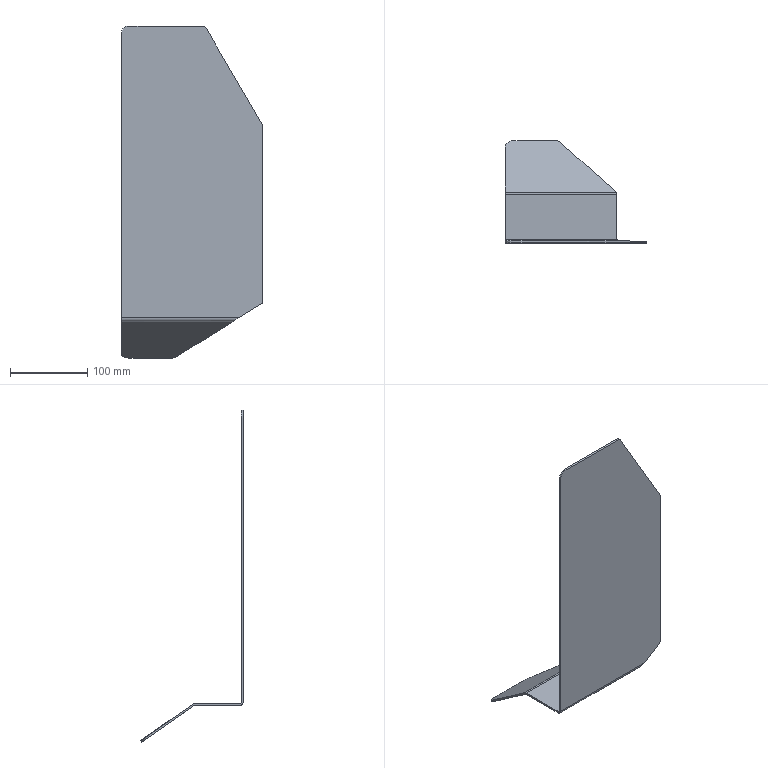Part | SolidWorks | features Fillet 2, FlatPattern 1, ICE 1, SMBaseFlange 1, SheetMetal 1 | 1 solid | 30 faces | box 183 x 132.321 x 429 mm | volume 188831 mm3 | plane 18 | cylinder 10 | spline 2 | commonest cylinder face diameters 10 x4 5 x2 9.6 x2 20 x2
STEP:
#1=CARTESIAN_POINT('',(-24.691,131.,-429.));
#2=VERTEX_POINT('',#1);
#3=CARTESIAN_POINT('',(-81.5,131.,-429.));
#4=VERTEX_POINT('',#3);
#5=CARTESIAN_POINT('',(91.5,131.,-429.));
#6=DIRECTION('',(-1.,0.,0.));
#7=VECTOR('',#6,1000.);
#8=LINE('',#5,#7);
#9=EDGE_CURVE('',#2,#4,#8,.T.);
#10=ORIENTED_EDGE('',*,*,#9,.F.);
#11=CARTESIAN_POINT('',(-21.015,129.681,-428.075));
#12=VERTEX_POINT('',#11);
#13=CARTESIAN_POINT('',(-24.691,126.907,-426.129));
#14=DIRECTION('',(0.,-0.5743,-0.8187));
#15=DIRECTION('',(0.,-0.8187,0.5743));
#16=AXIS2_PLACEMENT_3D('',#13,#14,#15);
#17=CIRCLE('',#16,5.);
#18=EDGE_CURVE('',#2,#12,#17,.T.);
#19=ORIENTED_EDGE('',*,*,#18,.T.);
#20=CARTESIAN_POINT('',(52.237,64.646,-382.453));
#21=VERTEX_POINT('',#20);
#22=CARTESIAN_POINT('',(70.673,48.278,-370.971));
#23=DIRECTION('',(0.6779,-0.6018,0.4222));
#24=VECTOR('',#23,1000.);
#25=LINE('',#22,#24);
#26=EDGE_CURVE('',#12,#21,#25,.T.);
#27=ORIENTED_EDGE('',*,*,#26,.T.);
#28=CARTESIAN_POINT('',(-91.5,64.646,-382.453));
#29=VERTEX_POINT('',#28);
#30=CARTESIAN_POINT('',(91.5,64.646,-382.453));
#31=DIRECTION('',(-1.,0.,0.));
#32=VECTOR('',#31,1000.);
#33=LINE('',#30,#32);
#34=EDGE_CURVE('',#21,#29,#33,.T.);
#35=ORIENTED_EDGE('',*,*,#34,.T.);
#36=CARTESIAN_POINT('',(-91.5,122.813,-423.257));
#37=VERTEX_POINT('',#36);
#38=CARTESIAN_POINT('',(-91.5,64.,-382.));
#39=DIRECTION('',(0.,0.8187,-0.5743));
#40=VECTOR('',#39,1000.);
#41=LINE('',#38,#40);
#42=EDGE_CURVE('',#29,#37,#41,.T.);
#43=ORIENTED_EDGE('',*,*,#42,.T.);
#44=CARTESIAN_POINT('',(-81.5,122.813,-423.257));
#45=DIRECTION('',(0.,-0.5743,-0.8187));
#46=DIRECTION('',(0.,-0.8187,0.5743));
#47=AXIS2_PLACEMENT_3D('',#44,#45,#46);
#48=CIRCLE('',#47,10.);
#49=EDGE_CURVE('',#37,#4,#48,.T.);
#50=ORIENTED_EDGE('',*,*,#49,.T.);
#51=EDGE_LOOP('',(#10,#19,#27,#35,#43,#50));
#52=FACE_OUTER_BOUND('',#51,.T.);
#53=CARTESIAN_POINT('',(91.5,64.,-382.));
#54=DIRECTION('',(0.,0.5743,0.8187));
#55=DIRECTION('',(0.,-0.8187,0.5743));
#56=AXIS2_PLACEMENT_3D('',#53,#54,#55);
#57=PLANE('',#56);
#58=ADVANCED_FACE('',(#52),#57,.F.);
#59=CARTESIAN_POINT('',(-24.691,132.321,-427.117));
#60=VERTEX_POINT('',#59);
#61=CARTESIAN_POINT('',(-81.5,132.321,-427.117));
#62=VERTEX_POINT('',#61);
#63=CARTESIAN_POINT('',(91.5,132.321,-427.117));
#64=DIRECTION('',(-1.,0.,0.));
#65=VECTOR('',#64,1000.);
#66=LINE('',#63,#65);
#67=EDGE_CURVE('',#60,#62,#66,.T.);
#68=ORIENTED_EDGE('',*,*,#67,.F.);
#69=CARTESIAN_POINT('',(-24.691,132.321,-427.117));
#70=DIRECTION('',(0.,-0.5743,-0.8187));
#71=VECTOR('',#70,1000.);
#72=LINE('',#69,#71);
#73=EDGE_CURVE('',#60,#2,#72,.T.);
#74=ORIENTED_EDGE('',*,*,#73,.T.);
#75=ORIENTED_EDGE('',*,*,#9,.T.);
#76=CARTESIAN_POINT('',(-81.5,132.321,-427.117));
#77=DIRECTION('',(0.,0.5743,0.8187));
#78=VECTOR('',#77,1000.);
#79=LINE('',#76,#78);
#80=EDGE_CURVE('',#4,#62,#79,.T.);
#81=ORIENTED_EDGE('',*,*,#80,.T.);
#82=EDGE_LOOP('',(#68,#74,#75,#81));
#83=FACE_OUTER_BOUND('',#82,.T.);
#84=CARTESIAN_POINT('',(91.5,132.321,-427.117));
#85=DIRECTION('',(0.,0.8187,-0.5743));
#86=DIRECTION('',(0.,0.5743,0.8187));
#87=AXIS2_PLACEMENT_3D('',#84,#85,#86);
#88=PLANE('',#87);
#89=ADVANCED_FACE('',(#83),#88,.T.);
#90=CARTESIAN_POINT('',(-21.015,131.002,-426.192));
#91=VERTEX_POINT('',#90);
#92=CARTESIAN_POINT('',(52.237,65.967,-380.57));
#93=VERTEX_POINT('',#92);
#94=CARTESIAN_POINT('',(70.673,49.599,-369.088));
#95=DIRECTION('',(0.6779,-0.6018,0.4222));
#96=VECTOR('',#95,1000.);
#97=LINE('',#94,#96);
#98=EDGE_CURVE('',#91,#93,#97,.T.);
#99=ORIENTED_EDGE('',*,*,#98,.F.);
#100=CARTESIAN_POINT('',(-24.691,128.228,-424.246));
#101=DIRECTION('',(0.,0.5743,0.8187));
#102=DIRECTION('',(0.,-0.8187,0.5743));
#103=AXIS2_PLACEMENT_3D('',#100,#101,#102);
#104=CIRCLE('',#103,5.);
#105=EDGE_CURVE('',#91,#60,#104,.T.);
#106=ORIENTED_EDGE('',*,*,#105,.T.);
#107=ORIENTED_EDGE('',*,*,#67,.T.);
#108=CARTESIAN_POINT('',(-91.5,124.134,-421.374));
#109=VERTEX_POINT('',#108);
#110=CARTESIAN_POINT('',(-81.5,124.134,-421.374));
#111=DIRECTION('',(0.,0.5743,0.8187));
#112=DIRECTION('',(0.,-0.8187,0.5743));
#113=AXIS2_PLACEMENT_3D('',#110,#111,#112);
#114=CIRCLE('',#113,10.);
#115=EDGE_CURVE('',#62,#109,#114,.T.);
#116=ORIENTED_EDGE('',*,*,#115,.T.);
#117=CARTESIAN_POINT('',(-91.5,65.967,-380.57));
#118=VERTEX_POINT('',#117);
#119=CARTESIAN_POINT('',(-91.5,65.321,-380.117));
#120=DIRECTION('',(0.,0.8187,-0.5743));
#121=VECTOR('',#120,1000.);
#122=LINE('',#119,#121);
#123=EDGE_CURVE('',#118,#109,#122,.T.);
#124=ORIENTED_EDGE('',*,*,#123,.F.);
#125=CARTESIAN_POINT('',(91.5,65.967,-380.57));
#126=DIRECTION('',(-1.,0.,0.));
#127=VECTOR('',#126,1000.);
#128=LINE('',#125,#127);
#129=EDGE_CURVE('',#93,#118,#128,.T.);
#130=ORIENTED_EDGE('',*,*,#129,.F.);
#131=EDGE_LOOP('',(#99,#106,#107,#116,#124,#130));
#132=FACE_OUTER_BOUND('',#131,.T.);
#133=CARTESIAN_POINT('',(91.5,65.321,-380.117));
#134=DIRECTION('',(0.,0.5743,0.8187));
#135=DIRECTION('',(0.,-0.8187,0.5743));
#136=AXIS2_PLACEMENT_3D('',#133,#134,#135);
#137=PLANE('',#136);
#138=ADVANCED_FACE('',(#132),#137,.T.);
#139=CARTESIAN_POINT('',(52.965,63.211,-379.7));
#140=VERTEX_POINT('',#139);
#141=CARTESIAN_POINT('',(-91.5,63.211,-379.7));
#142=VERTEX_POINT('',#141);
#143=CARTESIAN_POINT('',(91.5,63.211,-379.7));
#144=DIRECTION('',(-1.,0.,0.));
#145=VECTOR('',#144,1000.);
#146=LINE('',#143,#145);
#147=EDGE_CURVE('',#140,#142,#146,.T.);
#148=ORIENTED_EDGE('',*,*,#147,.F.);
#149=CARTESIAN_POINT('',(52.237,65.967,-380.57));
#150=CARTESIAN_POINT('',(52.714,65.153,-379.999));
#151=CARTESIAN_POINT('',(52.965,64.205,-379.7));
#152=CARTESIAN_POINT('',(52.965,63.211,-379.7));
#153=(BOUNDED_CURVE()B_SPLINE_CURVE(3,(#149,#150,#151,#152),.UNSPECIFIED.,.F.,.F.)B_SPLINE_CURVE_WITH_KNOTS((4,4),(2.53,3.142),.UNSPECIFIED.)CURVE()GEOMETRIC_REPRESENTATION_ITEM()RATIONAL_B_SPLINE_CURVE((1.,0.9691,0.9691,1.))REPRESENTATION_ITEM(''));
#154=EDGE_CURVE('',#93,#140,#153,.T.);
#155=ORIENTED_EDGE('',*,*,#154,.F.);
#156=ORIENTED_EDGE('',*,*,#129,.T.);
#157=CARTESIAN_POINT('',(-91.5,63.211,-384.5));
#158=DIRECTION('',(-1.,0.,0.));
#159=DIRECTION('',(0.,0.,-1.));
#160=AXIS2_PLACEMENT_3D('',#157,#158,#159);
#161=CIRCLE('',#160,4.8);
#162=EDGE_CURVE('',#142,#118,#161,.T.);
#163=ORIENTED_EDGE('',*,*,#162,.F.);
#164=EDGE_LOOP('',(#148,#155,#156,#163));
#165=FACE_OUTER_BOUND('',#164,.T.);
#166=CARTESIAN_POINT('',(91.5,63.211,-384.5));
#167=DIRECTION('',(-1.,0.,0.));
#168=DIRECTION('',(0.,0.,1.));
#169=AXIS2_PLACEMENT_3D('',#166,#167,#168);
#170=CYLINDRICAL_SURFACE('',#169,4.8);
#171=ADVANCED_FACE('',(#165),#170,.T.);
#172=CARTESIAN_POINT('',(52.965,4.8,-379.7));
#173=VERTEX_POINT('',#172);
#174=CARTESIAN_POINT('',(-91.5,4.8,-379.7));
#175=VERTEX_POINT('',#174);
#176=CARTESIAN_POINT('',(91.5,4.8,-379.7));
#177=DIRECTION('',(-1.,0.,0.));
#178=VECTOR('',#177,1000.);
#179=LINE('',#176,#178);
#180=EDGE_CURVE('',#173,#175,#179,.T.);
#181=ORIENTED_EDGE('',*,*,#180,.F.);
#182=CARTESIAN_POINT('',(52.965,0.,-379.7));
#183=DIRECTION('',(0.,-1.,0.));
#184=VECTOR('',#183,1000.);
#185=LINE('',#182,#184);
#186=EDGE_CURVE('',#140,#173,#185,.T.);
#187=ORIENTED_EDGE('',*,*,#186,.F.);
#188=ORIENTED_EDGE('',*,*,#147,.T.);
#189=CARTESIAN_POINT('',(-91.5,0.,-379.7));
#190=DIRECTION('',(0.,1.,0.));
#191=VECTOR('',#190,1000.);
#192=LINE('',#189,#191);
#193=EDGE_CURVE('',#175,#142,#192,.T.);
#194=ORIENTED_EDGE('',*,*,#193,.F.);
#195=EDGE_LOOP('',(#181,#187,#188,#194));
#196=FACE_OUTER_BOUND('',#195,.T.);
#197=CARTESIAN_POINT('',(91.5,0.,-379.7));
#198=DIRECTION('',(0.,0.,1.));
#199=DIRECTION('',(1.,0.,0.));
#200=AXIS2_PLACEMENT_3D('',#197,#198,#199);
#201=PLANE('',#200);
#202=ADVANCED_FACE('',(#196),#201,.T.);
#203=CARTESIAN_POINT('',(60.672,2.3,-377.2));
#204=VERTEX_POINT('',#203);
#205=CARTESIAN_POINT('',(-91.5,2.3,-377.2));
#206=VERTEX_POINT('',#205);
#207=CARTESIAN_POINT('',(91.5,2.3,-377.2));
#208=DIRECTION('',(-1.,0.,0.));
#209=VECTOR('',#208,1000.);
#210=LINE('',#207,#209);
#211=EDGE_CURVE('',#204,#206,#210,.T.);
#212=ORIENTED_EDGE('',*,*,#211,.F.);
#213=CARTESIAN_POINT('',(52.965,4.8,-379.7));
#214=CARTESIAN_POINT('',(52.965,3.336,-379.7));
#215=CARTESIAN_POINT('',(56.157,2.3,-378.664));
#216=CARTESIAN_POINT('',(60.672,2.3,-377.2));
#217=(BOUNDED_CURVE()B_SPLINE_CURVE(3,(#213,#214,#215,#216),.UNSPECIFIED.,.F.,.F.)B_SPLINE_CURVE_WITH_KNOTS((4,4),(0.,1.571),.UNSPECIFIED.)CURVE()GEOMETRIC_REPRESENTATION_ITEM()RATIONAL_B_SPLINE_CURVE((1.,0.8047,0.8047,1.))REPRESENTATION_ITEM(''));
#218=EDGE_CURVE('',#173,#204,#217,.T.);
#219=ORIENTED_EDGE('',*,*,#218,.F.);
#220=ORIENTED_EDGE('',*,*,#180,.T.);
#221=CARTESIAN_POINT('',(-91.5,4.8,-377.2));
#222=DIRECTION('',(1.,0.,0.));
#223=DIRECTION('',(0.,0.,-1.));
#224=AXIS2_PLACEMENT_3D('',#221,#222,#223);
#225=CIRCLE('',#224,2.5);
#226=EDGE_CURVE('',#206,#175,#225,.T.);
#227=ORIENTED_EDGE('',*,*,#226,.F.);
#228=EDGE_LOOP('',(#212,#219,#220,#227));
#229=FACE_OUTER_BOUND('',#228,.T.);
#230=CARTESIAN_POINT('',(91.5,4.8,-377.2));
#231=DIRECTION('',(-1.,0.,0.));
#232=DIRECTION('',(0.,0.,1.));
#233=AXIS2_PLACEMENT_3D('',#230,#231,#232);
#234=CYLINDRICAL_SURFACE('',#233,2.5);
#235=ADVANCED_FACE('',(#229),#234,.F.);
#236=CARTESIAN_POINT('',(91.5,2.3,-129.65));
#237=VERTEX_POINT('',#236);
#238=CARTESIAN_POINT('',(91.5,2.3,-355.224));
#239=VERTEX_POINT('',#238);
#240=CARTESIAN_POINT('',(91.5,2.3,0.));
#241=DIRECTION('',(0.,0.,-1.));
#242=VECTOR('',#241,1000.);
#243=LINE('',#240,#242);
#244=EDGE_CURVE('',#237,#239,#243,.T.);
#245=ORIENTED_EDGE('',*,*,#244,.T.);
#246=CARTESIAN_POINT('',(89.143,2.3,-359.468));
#247=VERTEX_POINT('',#246);
#248=CARTESIAN_POINT('',(86.5,2.3,-355.224));
#249=DIRECTION('',(0.,1.,0.));
#250=DIRECTION('',(0.,0.,1.));
#251=AXIS2_PLACEMENT_3D('',#248,#249,#250);
#252=CIRCLE('',#251,5.);
#253=EDGE_CURVE('',#239,#247,#252,.T.);
#254=ORIENTED_EDGE('',*,*,#253,.T.);
#255=CARTESIAN_POINT('',(252.15,2.3,-257.946));
#256=DIRECTION('',(0.8488,0.,0.5287));
#257=VECTOR('',#256,1000.);
#258=LINE('',#255,#257);
#259=EDGE_CURVE('',#204,#247,#258,.T.);
#260=ORIENTED_EDGE('',*,*,#259,.F.);
#261=ORIENTED_EDGE('',*,*,#211,.T.);
#262=CARTESIAN_POINT('',(-91.5,2.3,-10.));
#263=VERTEX_POINT('',#262);
#264=CARTESIAN_POINT('',(-91.5,2.3,0.));
#265=DIRECTION('',(0.,0.,-1.));
#266=VECTOR('',#265,1000.);
#267=LINE('',#264,#266);
#268=EDGE_CURVE('',#263,#206,#267,.T.);
#269=ORIENTED_EDGE('',*,*,#268,.F.);
#270=CARTESIAN_POINT('',(-81.5,2.3,0.));
#271=VERTEX_POINT('',#270);
#272=CARTESIAN_POINT('',(-81.5,2.3,-10.));
#273=DIRECTION('',(0.,1.,0.));
#274=DIRECTION('',(0.,0.,1.));
#275=AXIS2_PLACEMENT_3D('',#272,#273,#274);
#276=CIRCLE('',#275,10.);
#277=EDGE_CURVE('',#263,#271,#276,.T.);
#278=ORIENTED_EDGE('',*,*,#277,.T.);
#279=CARTESIAN_POINT('',(13.631,2.3,0.));
#280=VERTEX_POINT('',#279);
#281=CARTESIAN_POINT('',(91.5,2.3,0.));
#282=DIRECTION('',(-1.,0.,0.));
#283=VECTOR('',#282,1000.);
#284=LINE('',#281,#283);
#285=EDGE_CURVE('',#280,#271,#284,.T.);
#286=ORIENTED_EDGE('',*,*,#285,.F.);
#287=CARTESIAN_POINT('',(17.948,2.3,-2.477));
#288=VERTEX_POINT('',#287);
#289=CARTESIAN_POINT('',(13.631,2.3,-5.));
#290=DIRECTION('',(0.,1.,0.));
#291=DIRECTION('',(0.,0.,1.));
#292=AXIS2_PLACEMENT_3D('',#289,#290,#291);
#293=CIRCLE('',#292,5.);
#294=EDGE_CURVE('',#280,#288,#293,.T.);
#295=ORIENTED_EDGE('',*,*,#294,.T.);
#296=CARTESIAN_POINT('',(90.817,2.3,-127.127));
#297=VERTEX_POINT('',#296);
#298=CARTESIAN_POINT('',(35.603,2.3,-32.677));
#299=DIRECTION('',(-0.5047,0.,0.8633));
#300=VECTOR('',#299,1000.);
#301=LINE('',#298,#300);
#302=EDGE_CURVE('',#297,#288,#301,.T.);
#303=ORIENTED_EDGE('',*,*,#302,.F.);
#304=CARTESIAN_POINT('',(86.5,2.3,-129.65));
#305=DIRECTION('',(0.,1.,0.));
#306=DIRECTION('',(0.,0.,1.));
#307=AXIS2_PLACEMENT_3D('',#304,#305,#306);
#308=CIRCLE('',#307,5.);
#309=EDGE_CURVE('',#297,#237,#308,.T.);
#310=ORIENTED_EDGE('',*,*,#309,.T.);
#311=EDGE_LOOP('',(#245,#254,#260,#261,#269,#278,#286,#295,#303,#310));
#312=FACE_OUTER_BOUND('',#311,.T.);
#313=CARTESIAN_POINT('',(91.5,2.3,0.));
#314=DIRECTION('',(0.,1.,0.));
#315=DIRECTION('',(0.,0.,1.));
#316=AXIS2_PLACEMENT_3D('',#313,#314,#315);
#317=PLANE('',#316);
#318=ADVANCED_FACE('',(#312),#317,.T.);
#319=CARTESIAN_POINT('',(13.631,0.,0.));
#320=VERTEX_POINT('',#319);
#321=CARTESIAN_POINT('',(-81.5,0.,0.));
#322=VERTEX_POINT('',#321);
#323=CARTESIAN_POINT('',(91.5,0.,0.));
#324=DIRECTION('',(-1.,0.,0.));
#325=VECTOR('',#324,1000.);
#326=LINE('',#323,#325);
#327=EDGE_CURVE('',#320,#322,#326,.T.);
#328=ORIENTED_EDGE('',*,*,#327,.F.);
#329=CARTESIAN_POINT('',(13.631,0.,0.));
#330=DIRECTION('',(0.,1.,0.));
#331=VECTOR('',#330,1000.);
#332=LINE('',#329,#331);
#333=EDGE_CURVE('',#320,#280,#332,.T.);
#334=ORIENTED_EDGE('',*,*,#333,.T.);
#335=ORIENTED_EDGE('',*,*,#285,.T.);
#336=CARTESIAN_POINT('',(-81.5,0.,0.));
#337=DIRECTION('',(0.,-1.,0.));
#338=VECTOR('',#337,1000.);
#339=LINE('',#336,#338);
#340=EDGE_CURVE('',#271,#322,#339,.T.);
#341=ORIENTED_EDGE('',*,*,#340,.T.);
#342=EDGE_LOOP('',(#328,#334,#335,#341));
#343=FACE_OUTER_BOUND('',#342,.T.);
#344=CARTESIAN_POINT('',(91.5,0.,0.));
#345=DIRECTION('',(0.,0.,1.));
#346=DIRECTION('',(1.,0.,0.));
#347=AXIS2_PLACEMENT_3D('',#344,#345,#346);
#348=PLANE('',#347);
#349=ADVANCED_FACE('',(#343),#348,.T.);
#350=CARTESIAN_POINT('',(60.672,0.,-377.2));
#351=VERTEX_POINT('',#350);
#352=CARTESIAN_POINT('',(89.143,0.,-359.468));
#353=VERTEX_POINT('',#352);
#354=CARTESIAN_POINT('',(252.15,0.,-257.946));
#355=DIRECTION('',(0.8488,0.,0.5287));
#356=VECTOR('',#355,1000.);
#357=LINE('',#354,#356);
#358=EDGE_CURVE('',#351,#353,#357,.T.);
#359=ORIENTED_EDGE('',*,*,#358,.T.);
#360=CARTESIAN_POINT('',(91.5,0.,-355.224));
#361=VERTEX_POINT('',#360);
#362=CARTESIAN_POINT('',(86.5,0.,-355.224));
#363=DIRECTION('',(0.,-1.,0.));
#364=DIRECTION('',(0.,0.,1.));
#365=AXIS2_PLACEMENT_3D('',#362,#363,#364);
#366=CIRCLE('',#365,5.);
#367=EDGE_CURVE('',#353,#361,#366,.T.);
#368=ORIENTED_EDGE('',*,*,#367,.T.);
#369=CARTESIAN_POINT('',(91.5,0.,-129.65));
#370=VERTEX_POINT('',#369);
#371=CARTESIAN_POINT('',(91.5,0.,0.));
#372=DIRECTION('',(0.,0.,-1.));
#373=VECTOR('',#372,1000.);
#374=LINE('',#371,#373);
#375=EDGE_CURVE('',#370,#361,#374,.T.);
#376=ORIENTED_EDGE('',*,*,#375,.F.);
#377=CARTESIAN_POINT('',(90.817,0.,-127.127));
#378=VERTEX_POINT('',#377);
#379=CARTESIAN_POINT('',(86.5,0.,-129.65));
#380=DIRECTION('',(0.,-1.,0.));
#381=DIRECTION('',(0.,0.,1.));
#382=AXIS2_PLACEMENT_3D('',#379,#380,#381);
#383=CIRCLE('',#382,5.);
#384=EDGE_CURVE('',#370,#378,#383,.T.);
#385=ORIENTED_EDGE('',*,*,#384,.T.);
#386=CARTESIAN_POINT('',(17.948,0.,-2.477));
#387=VERTEX_POINT('',#386);
#388=CARTESIAN_POINT('',(35.603,0.,-32.677));
#389=DIRECTION('',(-0.5047,0.,0.8633));
#390=VECTOR('',#389,1000.);
#391=LINE('',#388,#390);
#392=EDGE_CURVE('',#378,#387,#391,.T.);
#393=ORIENTED_EDGE('',*,*,#392,.T.);
#394=CARTESIAN_POINT('',(13.631,0.,-5.));
#395=DIRECTION('',(0.,-1.,0.));
#396=DIRECTION('',(0.,0.,1.));
#397=AXIS2_PLACEMENT_3D('',#394,#395,#396);
#398=CIRCLE('',#397,5.);
#399=EDGE_CURVE('',#387,#320,#398,.T.);
#400=ORIENTED_EDGE('',*,*,#399,.T.);
#401=ORIENTED_EDGE('',*,*,#327,.T.);
#402=CARTESIAN_POINT('',(-91.5,0.,-10.));
#403=VERTEX_POINT('',#402);
#404=CARTESIAN_POINT('',(-81.5,0.,-10.));
#405=DIRECTION('',(0.,-1.,0.));
#406=DIRECTION('',(0.,0.,1.));
#407=AXIS2_PLACEMENT_3D('',#404,#405,#406);
#408=CIRCLE('',#407,10.);
#409=EDGE_CURVE('',#322,#403,#408,.T.);
#410=ORIENTED_EDGE('',*,*,#409,.T.);
#411=CARTESIAN_POINT('',(-91.5,0.,-377.2));
#412=VERTEX_POINT('',#411);
#413=CARTESIAN_POINT('',(-91.5,0.,0.));
#414=DIRECTION('',(0.,0.,-1.));
#415=VECTOR('',#414,1000.);
#416=LINE('',#413,#415);
#417=EDGE_CURVE('',#403,#412,#416,.T.);
#418=ORIENTED_EDGE('',*,*,#417,.T.);
#419=CARTESIAN_POINT('',(91.5,0.,-377.2));
#420=DIRECTION('',(-1.,0.,0.));
#421=VECTOR('',#420,1000.);
#422=LINE('',#419,#421);
#423=EDGE_CURVE('',#351,#412,#422,.T.);
#424=ORIENTED_EDGE('',*,*,#423,.F.);
#425=EDGE_LOOP('',(#359,#368,#376,#385,#393,#400,#401,#410,#418,#424));
#426=FACE_OUTER_BOUND('',#425,.T.);
#427=CARTESIAN_POINT('',(91.5,0.,0.));
#428=DIRECTION('',(0.,1.,0.));
#429=DIRECTION('',(0.,0.,1.));
#430=AXIS2_PLACEMENT_3D('',#427,#428,#429);
#431=PLANE('',#430);
#432=ADVANCED_FACE('',(#426),#431,.F.);
#433=CARTESIAN_POINT('',(52.965,4.8,-382.));
#434=VERTEX_POINT('',#433);
#435=CARTESIAN_POINT('',(52.965,4.8,-382.));
#436=CARTESIAN_POINT('',(52.965,1.988,-382.));
#437=CARTESIAN_POINT('',(56.157,0.,-380.012));
#438=CARTESIAN_POINT('',(60.672,0.,-377.2));
#439=(BOUNDED_CURVE()B_SPLINE_CURVE(3,(#435,#436,#437,#438),.UNSPECIFIED.,.F.,.F.)B_SPLINE_CURVE_WITH_KNOTS((4,4),(0.,1.571),.UNSPECIFIED.)CURVE()GEOMETRIC_REPRESENTATION_ITEM()RATIONAL_B_SPLINE_CURVE((1.,0.8047,0.8047,1.))REPRESENTATION_ITEM(''));
#440=EDGE_CURVE('',#434,#351,#439,.T.);
#441=ORIENTED_EDGE('',*,*,#440,.T.);
#442=ORIENTED_EDGE('',*,*,#423,.T.);
#443=CARTESIAN_POINT('',(-91.5,4.8,-382.));
#444=VERTEX_POINT('',#443);
#445=CARTESIAN_POINT('',(-91.5,4.8,-377.2));
#446=DIRECTION('',(1.,0.,0.));
#447=DIRECTION('',(0.,0.,1.));
#448=AXIS2_PLACEMENT_3D('',#445,#446,#447);
#449=CIRCLE('',#448,4.8);
#450=EDGE_CURVE('',#412,#444,#449,.T.);
#451=ORIENTED_EDGE('',*,*,#450,.T.);
#452=CARTESIAN_POINT('',(91.5,4.8,-382.));
#453=DIRECTION('',(-1.,0.,0.));
#454=VECTOR('',#453,1000.);
#455=LINE('',#452,#454);
#456=EDGE_CURVE('',#434,#444,#455,.T.);
#457=ORIENTED_EDGE('',*,*,#456,.F.);
#458=EDGE_LOOP('',(#441,#442,#451,#457));
#459=FACE_OUTER_BOUND('',#458,.T.);
#460=CARTESIAN_POINT('',(91.5,4.8,-377.2));
#461=DIRECTION('',(-1.,0.,0.));
#462=DIRECTION('',(0.,0.,1.));
#463=AXIS2_PLACEMENT_3D('',#460,#461,#462);
#464=CYLINDRICAL_SURFACE('',#463,4.8);
#465=ADVANCED_FACE('',(#459),#464,.T.);
#466=CARTESIAN_POINT('',(52.965,63.211,-382.));
#467=VERTEX_POINT('',#466);
#468=CARTESIAN_POINT('',(52.965,0.,-382.));
#469=DIRECTION('',(0.,-1.,0.));
#470=VECTOR('',#469,1000.);
#471=LINE('',#468,#470);
#472=EDGE_CURVE('',#467,#434,#471,.T.);
#473=ORIENTED_EDGE('',*,*,#472,.T.);
#474=ORIENTED_EDGE('',*,*,#456,.T.);
#475=CARTESIAN_POINT('',(-91.5,63.211,-382.));
#476=VERTEX_POINT('',#475);
#477=CARTESIAN_POINT('',(-91.5,0.,-382.));
#478=DIRECTION('',(0.,1.,0.));
#479=VECTOR('',#478,1000.);
#480=LINE('',#477,#479);
#481=EDGE_CURVE('',#444,#476,#480,.T.);
#482=ORIENTED_EDGE('',*,*,#481,.T.);
#483=CARTESIAN_POINT('',(91.5,63.211,-382.));
#484=DIRECTION('',(-1.,0.,0.));
#485=VECTOR('',#484,1000.);
#486=LINE('',#483,#485);
#487=EDGE_CURVE('',#467,#476,#486,.T.);
#488=ORIENTED_EDGE('',*,*,#487,.F.);
#489=EDGE_LOOP('',(#473,#474,#482,#488));
#490=FACE_OUTER_BOUND('',#489,.T.);
#491=CARTESIAN_POINT('',(91.5,0.,-382.));
#492=DIRECTION('',(0.,0.,1.));
#493=DIRECTION('',(1.,0.,0.));
#494=AXIS2_PLACEMENT_3D('',#491,#492,#493);
#495=PLANE('',#494);
#496=ADVANCED_FACE('',(#490),#495,.F.);
#497=CARTESIAN_POINT('',(52.237,64.646,-382.453));
#498=CARTESIAN_POINT('',(52.714,64.222,-382.156));
#499=CARTESIAN_POINT('',(52.965,63.728,-382.));
#500=CARTESIAN_POINT('',(52.965,63.211,-382.));
#501=(BOUNDED_CURVE()B_SPLINE_CURVE(3,(#497,#498,#499,#500),.UNSPECIFIED.,.F.,.F.)B_SPLINE_CURVE_WITH_KNOTS((4,4),(2.53,3.142),.UNSPECIFIED.)CURVE()GEOMETRIC_REPRESENTATION_ITEM()RATIONAL_B_SPLINE_CURVE((1.,0.9691,0.9691,1.))REPRESENTATION_ITEM(''));
#502=EDGE_CURVE('',#21,#467,#501,.T.);
#503=ORIENTED_EDGE('',*,*,#502,.T.);
#504=ORIENTED_EDGE('',*,*,#487,.T.);
#505=CARTESIAN_POINT('',(-91.5,63.211,-384.5));
#506=DIRECTION('',(-1.,0.,0.));
#507=DIRECTION('',(0.,0.,-1.));
#508=AXIS2_PLACEMENT_3D('',#505,#506,#507);
#509=CIRCLE('',#508,2.5);
#510=EDGE_CURVE('',#476,#29,#509,.T.);
#511=ORIENTED_EDGE('',*,*,#510,.T.);
#512=ORIENTED_EDGE('',*,*,#34,.F.);
#513=EDGE_LOOP('',(#503,#504,#511,#512));
#514=FACE_OUTER_BOUND('',#513,.T.);
#515=CARTESIAN_POINT('',(91.5,63.211,-384.5));
#516=DIRECTION('',(-1.,0.,0.));
#517=DIRECTION('',(0.,0.,1.));
#518=AXIS2_PLACEMENT_3D('',#515,#516,#517);
#519=CYLINDRICAL_SURFACE('',#518,2.5);
#520=ADVANCED_FACE('',(#514),#519,.F.);
#521=ORIENTED_EDGE('',*,*,#375,.T.);
#522=CARTESIAN_POINT('',(91.5,4.8,-355.224));
#523=DIRECTION('',(0.,1.,0.));
#524=VECTOR('',#523,1000.);
#525=LINE('',#522,#524);
#526=EDGE_CURVE('',#361,#239,#525,.T.);
#527=ORIENTED_EDGE('',*,*,#526,.T.);
#528=ORIENTED_EDGE('',*,*,#244,.F.);
#529=CARTESIAN_POINT('',(91.5,4.8,-129.65));
#530=DIRECTION('',(0.,-1.,0.));
#531=VECTOR('',#530,1000.);
#532=LINE('',#529,#531);
#533=EDGE_CURVE('',#237,#370,#532,.T.);
#534=ORIENTED_EDGE('',*,*,#533,.T.);
#535=EDGE_LOOP('',(#521,#527,#528,#534));
#536=FACE_OUTER_BOUND('',#535,.T.);
#537=CARTESIAN_POINT('',(91.5,4.8,-379.7));
#538=DIRECTION('',(1.,0.,0.));
#539=DIRECTION('',(0.,0.,-1.));
#540=AXIS2_PLACEMENT_3D('',#537,#538,#539);
#541=PLANE('',#540);
#542=ADVANCED_FACE('',(#536),#541,.T.);
#543=CARTESIAN_POINT('',(-91.5,4.8,-382.));
#544=DIRECTION('',(0.,0.,1.));
#545=VECTOR('',#544,1000.);
#546=LINE('',#543,#545);
#547=EDGE_CURVE('',#444,#175,#546,.T.);
#548=ORIENTED_EDGE('',*,*,#547,.F.);
#549=ORIENTED_EDGE('',*,*,#450,.F.);
#550=CARTESIAN_POINT('',(-91.5,2.3,-377.2));
#551=DIRECTION('',(0.,-1.,0.));
#552=VECTOR('',#551,1000.);
#553=LINE('',#550,#552);
#554=EDGE_CURVE('',#206,#412,#553,.T.);
#555=ORIENTED_EDGE('',*,*,#554,.F.);
#556=ORIENTED_EDGE('',*,*,#226,.T.);
#557=EDGE_LOOP('',(#548,#549,#555,#556));
#558=FACE_OUTER_BOUND('',#557,.T.);
#559=CARTESIAN_POINT('',(-91.5,4.8,-382.));
#560=DIRECTION('',(-1.,0.,0.));
#561=DIRECTION('',(0.,0.,1.));
#562=AXIS2_PLACEMENT_3D('',#559,#560,#561);
#563=PLANE('',#562);
#564=ADVANCED_FACE('',(#558),#563,.T.);
#565=ORIENTED_EDGE('',*,*,#481,.F.);
#566=ORIENTED_EDGE('',*,*,#547,.T.);
#567=ORIENTED_EDGE('',*,*,#193,.T.);
#568=CARTESIAN_POINT('',(-91.5,63.211,-379.7));
#569=DIRECTION('',(0.,0.,-1.));
#570=VECTOR('',#569,1000.);
#571=LINE('',#568,#570);
#572=EDGE_CURVE('',#142,#476,#571,.T.);
#573=ORIENTED_EDGE('',*,*,#572,.T.);
#574=EDGE_LOOP('',(#565,#566,#567,#573));
#575=FACE_OUTER_BOUND('',#574,.T.);
#576=CARTESIAN_POINT('',(-91.5,2.3,-377.2));
#577=DIRECTION('',(-1.,0.,0.));
#578=DIRECTION('',(0.,0.,1.));
#579=AXIS2_PLACEMENT_3D('',#576,#577,#578);
#580=PLANE('',#579);
#581=ADVANCED_FACE('',(#575),#580,.T.);
#582=CARTESIAN_POINT('',(-91.5,64.646,-382.453));
#583=DIRECTION('',(0.,0.5743,0.8187));
#584=VECTOR('',#583,1000.);
#585=LINE('',#582,#584);
#586=EDGE_CURVE('',#29,#118,#585,.T.);
#587=ORIENTED_EDGE('',*,*,#586,.F.);
#588=ORIENTED_EDGE('',*,*,#510,.F.);
#589=ORIENTED_EDGE('',*,*,#572,.F.);
#590=ORIENTED_EDGE('',*,*,#162,.T.);
#591=EDGE_LOOP('',(#587,#588,#589,#590));
#592=FACE_OUTER_BOUND('',#591,.T.);
#593=CARTESIAN_POINT('',(-91.5,64.646,-382.453));
#594=DIRECTION('',(-1.,0.,0.));
#595=DIRECTION('',(0.,0.,1.));
#596=AXIS2_PLACEMENT_3D('',#593,#594,#595);
#597=PLANE('',#596);
#598=ADVANCED_FACE('',(#592),#597,.T.);
#599=ORIENTED_EDGE('',*,*,#123,.T.);
#600=CARTESIAN_POINT('',(-91.5,123.634,-422.087));
#601=DIRECTION('',(0.,-0.5743,-0.8187));
#602=VECTOR('',#601,1000.);
#603=LINE('',#600,#602);
#604=EDGE_CURVE('',#109,#37,#603,.T.);
#605=ORIENTED_EDGE('',*,*,#604,.T.);
#606=ORIENTED_EDGE('',*,*,#42,.F.);
#607=ORIENTED_EDGE('',*,*,#586,.T.);
#608=EDGE_LOOP('',(#599,#605,#606,#607));
#609=FACE_OUTER_BOUND('',#608,.T.);
#610=CARTESIAN_POINT('',(-91.5,63.211,-379.7));
#611=DIRECTION('',(-1.,0.,0.));
#612=DIRECTION('',(0.,0.,1.));
#613=AXIS2_PLACEMENT_3D('',#610,#611,#612);
#614=PLANE('',#613);
#615=ADVANCED_FACE('',(#609),#614,.T.);
#616=ORIENTED_EDGE('',*,*,#417,.F.);
#617=CARTESIAN_POINT('',(-91.5,2.3,-10.));
#618=DIRECTION('',(0.,1.,0.));
#619=VECTOR('',#618,1000.);
#620=LINE('',#617,#619);
#621=EDGE_CURVE('',#403,#263,#620,.T.);
#622=ORIENTED_EDGE('',*,*,#621,.T.);
#623=ORIENTED_EDGE('',*,*,#268,.T.);
#624=ORIENTED_EDGE('',*,*,#554,.T.);
#625=EDGE_LOOP('',(#616,#622,#623,#624));
#626=FACE_OUTER_BOUND('',#625,.T.);
#627=CARTESIAN_POINT('',(-91.5,63.211,-384.5));
#628=DIRECTION('',(1.,0.,0.));
#629=DIRECTION('',(0.,0.,-1.));
#630=AXIS2_PLACEMENT_3D('',#627,#628,#629);
#631=PLANE('',#630);
#632=ADVANCED_FACE('',(#626),#631,.F.);
#633=ORIENTED_EDGE('',*,*,#259,.T.);
#634=CARTESIAN_POINT('',(89.143,2.3,-359.468));
#635=DIRECTION('',(0.,-1.,0.));
#636=VECTOR('',#635,1000.);
#637=LINE('',#634,#636);
#638=EDGE_CURVE('',#247,#353,#637,.T.);
#639=ORIENTED_EDGE('',*,*,#638,.T.);
#640=ORIENTED_EDGE('',*,*,#358,.F.);
#641=CARTESIAN_POINT('',(60.672,2.3,-377.2));
#642=DIRECTION('',(0.,-1.,0.));
#643=VECTOR('',#642,1000.);
#644=LINE('',#641,#643);
#645=EDGE_CURVE('',#204,#351,#644,.T.);
#646=ORIENTED_EDGE('',*,*,#645,.F.);
#647=EDGE_LOOP('',(#633,#639,#640,#646));
#648=FACE_OUTER_BOUND('',#647,.T.);
#649=CARTESIAN_POINT('',(252.15,2.3,-257.946));
#650=DIRECTION('',(-0.5287,0.,0.8488));
#651=DIRECTION('',(0.8488,0.,0.5287));
#652=AXIS2_PLACEMENT_3D('',#649,#650,#651);
#653=PLANE('',#652);
#654=ADVANCED_FACE('',(#648),#653,.F.);
#655=ORIENTED_EDGE('',*,*,#26,.F.);
#656=CARTESIAN_POINT('',(-21.015,129.681,-428.075));
#657=DIRECTION('',(0.,0.5743,0.8187));
#658=VECTOR('',#657,1000.);
#659=LINE('',#656,#658);
#660=EDGE_CURVE('',#12,#91,#659,.T.);
#661=ORIENTED_EDGE('',*,*,#660,.T.);
#662=ORIENTED_EDGE('',*,*,#98,.T.);
#663=CARTESIAN_POINT('',(52.237,64.646,-382.453));
#664=DIRECTION('',(0.,0.5743,0.8187));
#665=VECTOR('',#664,1000.);
#666=LINE('',#663,#665);
#667=EDGE_CURVE('',#21,#93,#666,.T.);
#668=ORIENTED_EDGE('',*,*,#667,.F.);
#669=EDGE_LOOP('',(#655,#661,#662,#668));
#670=FACE_OUTER_BOUND('',#669,.T.);
#671=CARTESIAN_POINT('',(70.673,48.278,-370.971));
#672=DIRECTION('',(-0.7352,-0.555,0.3893));
#673=DIRECTION('',(0.6779,-0.6018,0.4222));
#674=AXIS2_PLACEMENT_3D('',#671,#672,#673);
#675=PLANE('',#674);
#676=ADVANCED_FACE('',(#670),#675,.F.);
#677=CARTESIAN_POINT('',(52.965,63.211,-382.));
#678=DIRECTION('',(0.,0.,1.));
#679=VECTOR('',#678,1000.);
#680=LINE('',#677,#679);
#681=EDGE_CURVE('',#467,#140,#680,.T.);
#682=ORIENTED_EDGE('',*,*,#681,.F.);
#683=ORIENTED_EDGE('',*,*,#502,.F.);
#684=ORIENTED_EDGE('',*,*,#667,.T.);
#685=ORIENTED_EDGE('',*,*,#154,.T.);
#686=EDGE_LOOP('',(#682,#683,#684,#685));
#687=FACE_OUTER_BOUND('',#686,.T.);
#688=CARTESIAN_POINT('',(44.937,63.211,-389.3));
#689=CARTESIAN_POINT('',(44.937,63.211,-388.533));
#690=CARTESIAN_POINT('',(44.937,63.211,-387.767));
#691=CARTESIAN_POINT('',(44.937,63.211,-387.));
#692=CARTESIAN_POINT('',(44.937,72.811,-389.3));
#693=CARTESIAN_POINT('',(44.937,71.277,-388.533));
#694=CARTESIAN_POINT('',(44.937,69.744,-387.767));
#695=CARTESIAN_POINT('',(44.937,68.211,-387.));
#696=CARTESIAN_POINT('',(52.965,72.811,-379.7));
#697=CARTESIAN_POINT('',(52.965,71.277,-380.467));
#698=CARTESIAN_POINT('',(52.965,69.744,-381.233));
#699=CARTESIAN_POINT('',(52.965,68.211,-382.));
#700=CARTESIAN_POINT('',(52.965,63.211,-379.7));
#701=CARTESIAN_POINT('',(52.965,63.211,-380.467));
#702=CARTESIAN_POINT('',(52.965,63.211,-381.233));
#703=CARTESIAN_POINT('',(52.965,63.211,-382.));
#704=CARTESIAN_POINT('',(52.965,53.611,-379.7));
#705=CARTESIAN_POINT('',(52.965,55.144,-380.467));
#706=CARTESIAN_POINT('',(52.965,56.677,-381.233));
#707=CARTESIAN_POINT('',(52.965,58.211,-382.));
#708=CARTESIAN_POINT('',(44.937,53.611,-389.3));
#709=CARTESIAN_POINT('',(44.937,55.144,-388.533));
#710=CARTESIAN_POINT('',(44.937,56.677,-387.767));
#711=CARTESIAN_POINT('',(44.937,58.211,-387.));
#712=CARTESIAN_POINT('',(44.937,63.211,-389.3));
#713=CARTESIAN_POINT('',(44.937,63.211,-388.533));
#714=CARTESIAN_POINT('',(44.937,63.211,-387.767));
#715=CARTESIAN_POINT('',(44.937,63.211,-387.));
#716=(BOUNDED_SURFACE()B_SPLINE_SURFACE(3,3,((#688,#689,#690,#691),(#692,#693,#694,#695),(#696,#697,#698,#699),(#700,#701,#702,#703),(#704,#705,#706,#707),(#708,#709,#710,#711),(#712,#713,#714,#715)),.UNSPECIFIED.,.T.,.F.,.F.)B_SPLINE_SURFACE_WITH_KNOTS((4,3,4),(4,4),(0.,0.5,1.),(0.,1.),.UNSPECIFIED.)GEOMETRIC_REPRESENTATION_ITEM()RATIONAL_B_SPLINE_SURFACE(((1.,1.,1.,1.),(0.3333,0.3333,0.3333,0.3333),(0.3333,0.3333,0.3333,0.3333),(1.,1.,1.,1.),(0.3333,0.3333,0.3333,0.3333),(0.3333,0.3333,0.3333,0.3333),(1.,1.,1.,1.)))REPRESENTATION_ITEM('')SURFACE());
#717=ADVANCED_FACE('',(#687),#716,.T.);
#718=CARTESIAN_POINT('',(52.965,4.8,-382.));
#719=DIRECTION('',(0.,0.,1.));
#720=VECTOR('',#719,1000.);
#721=LINE('',#718,#720);
#722=EDGE_CURVE('',#434,#173,#721,.T.);
#723=ORIENTED_EDGE('',*,*,#722,.F.);
#724=ORIENTED_EDGE('',*,*,#472,.F.);
#725=ORIENTED_EDGE('',*,*,#681,.T.);
#726=ORIENTED_EDGE('',*,*,#186,.T.);
#727=EDGE_LOOP('',(#723,#724,#725,#726));
#728=FACE_OUTER_BOUND('',#727,.T.);
#729=CARTESIAN_POINT('',(52.965,0.,-382.));
#730=DIRECTION('',(-1.,0.,0.));
#731=DIRECTION('',(0.,-1.,0.));
#732=AXIS2_PLACEMENT_3D('',#729,#730,#731);
#733=PLANE('',#732);
#734=ADVANCED_FACE('',(#728),#733,.F.);
#735=ORIENTED_EDGE('',*,*,#645,.T.);
#736=ORIENTED_EDGE('',*,*,#440,.F.);
#737=ORIENTED_EDGE('',*,*,#722,.T.);
#738=ORIENTED_EDGE('',*,*,#218,.T.);
#739=EDGE_LOOP('',(#735,#736,#737,#738));
#740=FACE_OUTER_BOUND('',#739,.T.);
#741=CARTESIAN_POINT('',(52.965,4.8,-379.7));
#742=CARTESIAN_POINT('',(52.965,4.8,-380.467));
#743=CARTESIAN_POINT('',(52.965,4.8,-381.233));
#744=CARTESIAN_POINT('',(52.965,4.8,-382.));
#745=CARTESIAN_POINT('',(52.965,-0.2,-379.7));
#746=CARTESIAN_POINT('',(52.965,-1.733,-380.467));
#747=CARTESIAN_POINT('',(52.965,-3.267,-381.233));
#748=CARTESIAN_POINT('',(52.965,-4.8,-382.));
#749=CARTESIAN_POINT('',(68.379,-0.2,-374.7));
#750=CARTESIAN_POINT('',(68.379,-1.733,-373.933));
#751=CARTESIAN_POINT('',(68.379,-3.267,-373.167));
#752=CARTESIAN_POINT('',(68.379,-4.8,-372.4));
#753=CARTESIAN_POINT('',(68.379,4.8,-374.7));
#754=CARTESIAN_POINT('',(68.379,4.8,-373.933));
#755=CARTESIAN_POINT('',(68.379,4.8,-373.167));
#756=CARTESIAN_POINT('',(68.379,4.8,-372.4));
#757=CARTESIAN_POINT('',(68.379,9.8,-374.7));
#758=CARTESIAN_POINT('',(68.379,11.333,-373.933));
#759=CARTESIAN_POINT('',(68.379,12.867,-373.167));
#760=CARTESIAN_POINT('',(68.379,14.4,-372.4));
#761=CARTESIAN_POINT('',(52.965,9.8,-379.7));
#762=CARTESIAN_POINT('',(52.965,11.333,-380.467));
#763=CARTESIAN_POINT('',(52.965,12.867,-381.233));
#764=CARTESIAN_POINT('',(52.965,14.4,-382.));
#765=CARTESIAN_POINT('',(52.965,4.8,-379.7));
#766=CARTESIAN_POINT('',(52.965,4.8,-380.467));
#767=CARTESIAN_POINT('',(52.965,4.8,-381.233));
#768=CARTESIAN_POINT('',(52.965,4.8,-382.));
#769=(BOUNDED_SURFACE()B_SPLINE_SURFACE(3,3,((#741,#742,#743,#744),(#745,#746,#747,#748),(#749,#750,#751,#752),(#753,#754,#755,#756),(#757,#758,#759,#760),(#761,#762,#763,#764),(#765,#766,#767,#768)),.UNSPECIFIED.,.T.,.F.,.F.)B_SPLINE_SURFACE_WITH_KNOTS((4,3,4),(4,4),(0.,0.5,1.),(0.,1.),.UNSPECIFIED.)GEOMETRIC_REPRESENTATION_ITEM()RATIONAL_B_SPLINE_SURFACE(((1.,1.,1.,1.),(0.3333,0.3333,0.3333,0.3333),(0.3333,0.3333,0.3333,0.3333),(1.,1.,1.,1.),(0.3333,0.3333,0.3333,0.3333),(0.3333,0.3333,0.3333,0.3333),(1.,1.,1.,1.)))REPRESENTATION_ITEM('')SURFACE());
#770=ADVANCED_FACE('',(#740),#769,.T.);
#771=ORIENTED_EDGE('',*,*,#392,.F.);
#772=CARTESIAN_POINT('',(90.817,2.3,-127.127));
#773=DIRECTION('',(0.,1.,0.));
#774=VECTOR('',#773,1000.);
#775=LINE('',#772,#774);
#776=EDGE_CURVE('',#378,#297,#775,.T.);
#777=ORIENTED_EDGE('',*,*,#776,.T.);
#778=ORIENTED_EDGE('',*,*,#302,.T.);
#779=CARTESIAN_POINT('',(17.948,2.3,-2.477));
#780=DIRECTION('',(0.,-1.,0.));
#781=VECTOR('',#780,1000.);
#782=LINE('',#779,#781);
#783=EDGE_CURVE('',#288,#387,#782,.T.);
#784=ORIENTED_EDGE('',*,*,#783,.T.);
#785=EDGE_LOOP('',(#771,#777,#778,#784));
#786=FACE_OUTER_BOUND('',#785,.T.);
#787=CARTESIAN_POINT('',(35.603,2.3,-32.677));
#788=DIRECTION('',(-0.8633,0.,-0.5047));
#789=DIRECTION('',(-0.5047,0.,0.8633));
#790=AXIS2_PLACEMENT_3D('',#787,#788,#789);
#791=PLANE('',#790);
#792=ADVANCED_FACE('',(#786),#791,.F.);
#793=ORIENTED_EDGE('',*,*,#409,.F.);
#794=ORIENTED_EDGE('',*,*,#340,.F.);
#795=ORIENTED_EDGE('',*,*,#277,.F.);
#796=ORIENTED_EDGE('',*,*,#621,.F.);
#797=EDGE_LOOP('',(#793,#794,#795,#796));
#798=FACE_OUTER_BOUND('',#797,.T.);
#799=CARTESIAN_POINT('',(-81.5,63.211,-10.));
#800=DIRECTION('',(0.,-1.,0.));
#801=DIRECTION('',(0.,0.,-1.));
#802=AXIS2_PLACEMENT_3D('',#799,#800,#801);
#803=CYLINDRICAL_SURFACE('',#802,10.);
#804=ADVANCED_FACE('',(#798),#803,.T.);
#805=ORIENTED_EDGE('',*,*,#115,.F.);
#806=ORIENTED_EDGE('',*,*,#80,.F.);
#807=ORIENTED_EDGE('',*,*,#49,.F.);
#808=ORIENTED_EDGE('',*,*,#604,.F.);
#809=EDGE_LOOP('',(#805,#806,#807,#808));
#810=FACE_OUTER_BOUND('',#809,.T.);
#811=CARTESIAN_POINT('',(-81.5,123.634,-422.087));
#812=DIRECTION('',(0.,-0.5743,-0.8187));
#813=DIRECTION('',(0.,0.8187,-0.5743));
#814=AXIS2_PLACEMENT_3D('',#811,#812,#813);
#815=CYLINDRICAL_SURFACE('',#814,10.);
#816=ADVANCED_FACE('',(#810),#815,.T.);
#817=ORIENTED_EDGE('',*,*,#18,.F.);
#818=ORIENTED_EDGE('',*,*,#73,.F.);
#819=ORIENTED_EDGE('',*,*,#105,.F.);
#820=ORIENTED_EDGE('',*,*,#660,.F.);
#821=EDGE_LOOP('',(#817,#818,#819,#820));
#822=FACE_OUTER_BOUND('',#821,.T.);
#823=CARTESIAN_POINT('',(-24.691,126.907,-426.129));
#824=DIRECTION('',(0.,-0.5743,-0.8187));
#825=DIRECTION('',(0.,0.8187,-0.5743));
#826=AXIS2_PLACEMENT_3D('',#823,#824,#825);
#827=CYLINDRICAL_SURFACE('',#826,5.);
#828=ADVANCED_FACE('',(#822),#827,.T.);
#829=ORIENTED_EDGE('',*,*,#253,.F.);
#830=ORIENTED_EDGE('',*,*,#526,.F.);
#831=ORIENTED_EDGE('',*,*,#367,.F.);
#832=ORIENTED_EDGE('',*,*,#638,.F.);
#833=EDGE_LOOP('',(#829,#830,#831,#832));
#834=FACE_OUTER_BOUND('',#833,.T.);
#835=CARTESIAN_POINT('',(86.5,2.3,-355.224));
#836=DIRECTION('',(0.,1.,0.));
#837=DIRECTION('',(0.,0.,1.));
#838=AXIS2_PLACEMENT_3D('',#835,#836,#837);
#839=CYLINDRICAL_SURFACE('',#838,5.);
#840=ADVANCED_FACE('',(#834),#839,.T.);
#841=ORIENTED_EDGE('',*,*,#309,.F.);
#842=ORIENTED_EDGE('',*,*,#776,.F.);
#843=ORIENTED_EDGE('',*,*,#384,.F.);
#844=ORIENTED_EDGE('',*,*,#533,.F.);
#845=EDGE_LOOP('',(#841,#842,#843,#844));
#846=FACE_OUTER_BOUND('',#845,.T.);
#847=CARTESIAN_POINT('',(86.5,4.8,-129.65));
#848=DIRECTION('',(0.,1.,0.));
#849=DIRECTION('',(0.,0.,1.));
#850=AXIS2_PLACEMENT_3D('',#847,#848,#849);
#851=CYLINDRICAL_SURFACE('',#850,5.);
#852=ADVANCED_FACE('',(#846),#851,.T.);
#853=ORIENTED_EDGE('',*,*,#294,.F.);
#854=ORIENTED_EDGE('',*,*,#333,.F.);
#855=ORIENTED_EDGE('',*,*,#399,.F.);
#856=ORIENTED_EDGE('',*,*,#783,.F.);
#857=EDGE_LOOP('',(#853,#854,#855,#856));
#858=FACE_OUTER_BOUND('',#857,.T.);
#859=CARTESIAN_POINT('',(13.631,2.3,-5.));
#860=DIRECTION('',(0.,1.,0.));
#861=DIRECTION('',(0.,0.,1.));
#862=AXIS2_PLACEMENT_3D('',#859,#860,#861);
#863=CYLINDRICAL_SURFACE('',#862,5.);
#864=ADVANCED_FACE('',(#858),#863,.T.);
#865=CLOSED_SHELL('',(#58,#89,#138,#171,#202,#235,#318,#349,#432,#465,#496,#520,#542,#564,#581,#598,#615,#632,#654,#676,#717,#734,#770,#792,#804,#816,#828,#840,#852,#864));
#866=MANIFOLD_SOLID_BREP('',#865);
#867=CARTESIAN_POINT('',(0.,0.,0.));
#868=DIRECTION('',(0.,0.,1.));
#869=DIRECTION('',(1.,0.,0.));
#870=AXIS2_PLACEMENT_3D('',#867,#868,#869);
#871=(LENGTH_UNIT()NAMED_UNIT(*)SI_UNIT(.MILLI.,.METRE.));
#872=UNCERTAINTY_MEASURE_WITH_UNIT(LENGTH_MEASURE(0.00001),#871,'','');
#873=(NAMED_UNIT(*)PLANE_ANGLE_UNIT()SI_UNIT($,.RADIAN.));
#874=(NAMED_UNIT(*)SI_UNIT($,.STERADIAN.)SOLID_ANGLE_UNIT());
#875=(GEOMETRIC_REPRESENTATION_CONTEXT(3)GLOBAL_UNCERTAINTY_ASSIGNED_CONTEXT((#872))GLOBAL_UNIT_ASSIGNED_CONTEXT((#871,#873,#874))REPRESENTATION_CONTEXT('',''));
#876=ADVANCED_BREP_SHAPE_REPRESENTATION('',(#866,#870),#875);